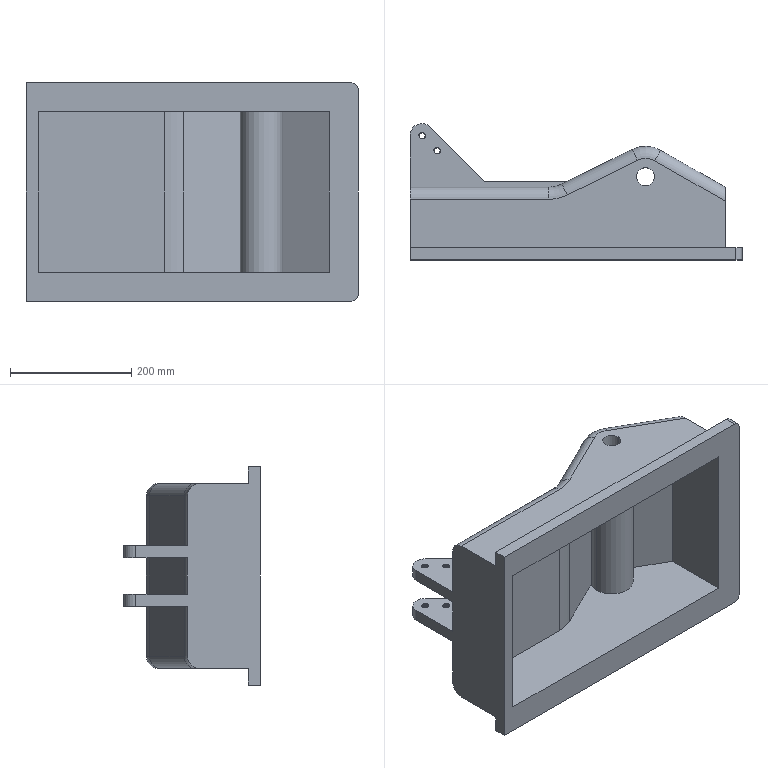Part | SolidWorks | 1 solid | 181 faces | box 547.5 x 225 x 360 mm | volume 8692071 mm3 | cylinder 132 | plane 33 | spline 12 | torus 4 | commonest cylinder face diameters 10 x112 40 x8 100 x4 70 x3 20 x2 30 x2